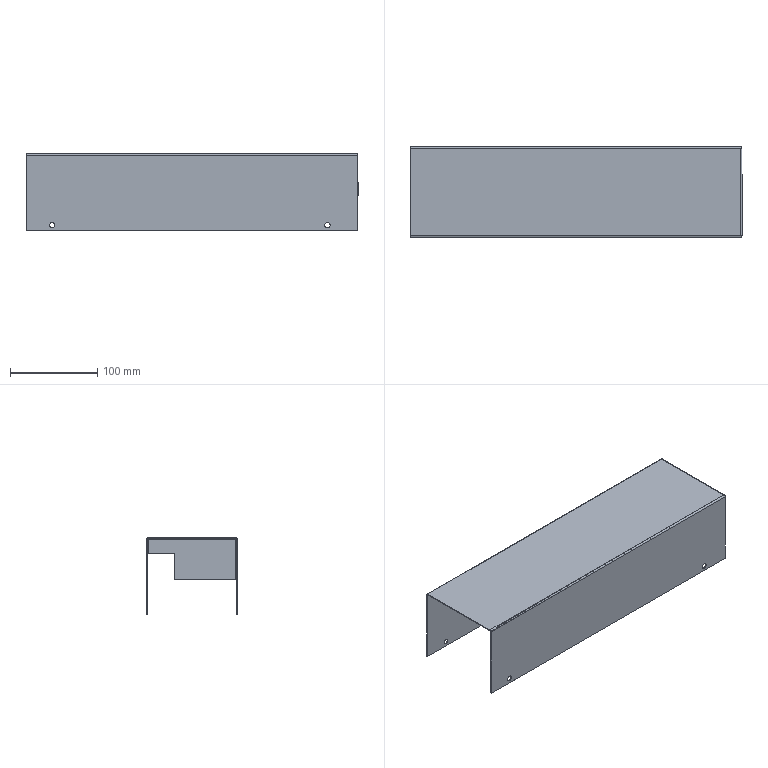Part | SolidWorks | features BaseBody 1 | 1 solid | 38 faces | box 380 x 104 x 88 mm | volume 108125 mm3 | plane 22 | cylinder 16 | commonest cylinder face diameters 6 x8 1.473 x3 3.473 x3 12 x2
STEP:
#1=CARTESIAN_POINT('',(332.,51.,-85.));
#2=VERTEX_POINT('',#1);
#3=CARTESIAN_POINT('',(332.,51.,-79.));
#4=VERTEX_POINT('',#3);
#5=CARTESIAN_POINT('',(332.,51.,-82.));
#6=DIRECTION('',(0.,1.,0.));
#7=DIRECTION('',(0.,0.,1.));
#8=AXIS2_PLACEMENT_3D('',#5,#6,#7);
#9=CIRCLE('',#8,3.);
#10=EDGE_CURVE('',#2,#4,#9,.T.);
#11=ORIENTED_EDGE('',*,*,#10,.F.);
#12=CARTESIAN_POINT('',(332.,52.,-85.));
#13=VERTEX_POINT('',#12);
#14=CARTESIAN_POINT('',(332.,-52.,-85.));
#15=DIRECTION('',(0.,1.,0.));
#16=VECTOR('',#15,1000.);
#17=LINE('',#14,#16);
#18=EDGE_CURVE('',#2,#13,#17,.T.);
#19=ORIENTED_EDGE('',*,*,#18,.T.);
#20=CARTESIAN_POINT('',(332.,52.,-79.));
#21=VERTEX_POINT('',#20);
#22=CARTESIAN_POINT('',(332.,52.,-82.));
#23=DIRECTION('',(0.,1.,0.));
#24=DIRECTION('',(0.,0.,1.));
#25=AXIS2_PLACEMENT_3D('',#22,#23,#24);
#26=CIRCLE('',#25,3.);
#27=EDGE_CURVE('',#13,#21,#26,.T.);
#28=ORIENTED_EDGE('',*,*,#27,.T.);
#29=CARTESIAN_POINT('',(332.,-52.,-79.));
#30=DIRECTION('',(0.,1.,0.));
#31=VECTOR('',#30,1000.);
#32=LINE('',#29,#31);
#33=EDGE_CURVE('',#4,#21,#32,.T.);
#34=ORIENTED_EDGE('',*,*,#33,.F.);
#35=EDGE_LOOP('',(#11,#19,#28,#34));
#36=FACE_OUTER_BOUND('',#35,.T.);
#37=CARTESIAN_POINT('',(332.,-52.,-82.));
#38=DIRECTION('',(0.,1.,0.));
#39=DIRECTION('',(0.,0.,1.));
#40=AXIS2_PLACEMENT_3D('',#37,#38,#39);
#41=CYLINDRICAL_SURFACE('',#40,3.);
#42=ADVANCED_FACE('',(#36),#41,.F.);
#43=CARTESIAN_POINT('',(17.,51.,-85.));
#44=VERTEX_POINT('',#43);
#45=CARTESIAN_POINT('',(17.,51.,-79.));
#46=VERTEX_POINT('',#45);
#47=CARTESIAN_POINT('',(17.,51.,-82.));
#48=DIRECTION('',(0.,1.,0.));
#49=DIRECTION('',(0.,0.,1.));
#50=AXIS2_PLACEMENT_3D('',#47,#48,#49);
#51=CIRCLE('',#50,3.);
#52=EDGE_CURVE('',#44,#46,#51,.T.);
#53=ORIENTED_EDGE('',*,*,#52,.F.);
#54=CARTESIAN_POINT('',(17.,52.,-85.));
#55=VERTEX_POINT('',#54);
#56=CARTESIAN_POINT('',(17.,-52.,-85.));
#57=DIRECTION('',(0.,1.,0.));
#58=VECTOR('',#57,1000.);
#59=LINE('',#56,#58);
#60=EDGE_CURVE('',#44,#55,#59,.T.);
#61=ORIENTED_EDGE('',*,*,#60,.T.);
#62=CARTESIAN_POINT('',(17.,52.,-79.));
#63=VERTEX_POINT('',#62);
#64=CARTESIAN_POINT('',(17.,52.,-82.));
#65=DIRECTION('',(0.,1.,0.));
#66=DIRECTION('',(0.,0.,1.));
#67=AXIS2_PLACEMENT_3D('',#64,#65,#66);
#68=CIRCLE('',#67,3.);
#69=EDGE_CURVE('',#55,#63,#68,.T.);
#70=ORIENTED_EDGE('',*,*,#69,.T.);
#71=CARTESIAN_POINT('',(17.,-52.,-79.));
#72=DIRECTION('',(0.,1.,0.));
#73=VECTOR('',#72,1000.);
#74=LINE('',#71,#73);
#75=EDGE_CURVE('',#46,#63,#74,.T.);
#76=ORIENTED_EDGE('',*,*,#75,.F.);
#77=EDGE_LOOP('',(#53,#61,#70,#76));
#78=FACE_OUTER_BOUND('',#77,.T.);
#79=CARTESIAN_POINT('',(17.,-52.,-82.));
#80=DIRECTION('',(0.,1.,0.));
#81=DIRECTION('',(0.,0.,1.));
#82=AXIS2_PLACEMENT_3D('',#79,#80,#81);
#83=CYLINDRICAL_SURFACE('',#82,3.);
#84=ADVANCED_FACE('',(#78),#83,.F.);
#85=CARTESIAN_POINT('',(17.,-52.,-85.));
#86=VERTEX_POINT('',#85);
#87=CARTESIAN_POINT('',(17.,-52.,-79.));
#88=VERTEX_POINT('',#87);
#89=CARTESIAN_POINT('',(17.,-52.,-82.));
#90=DIRECTION('',(0.,1.,0.));
#91=DIRECTION('',(0.,0.,1.));
#92=AXIS2_PLACEMENT_3D('',#89,#90,#91);
#93=CIRCLE('',#92,3.);
#94=EDGE_CURVE('',#86,#88,#93,.T.);
#95=ORIENTED_EDGE('',*,*,#94,.F.);
#96=CARTESIAN_POINT('',(17.,-51.,-85.));
#97=VERTEX_POINT('',#96);
#98=CARTESIAN_POINT('',(17.,-52.,-85.));
#99=DIRECTION('',(0.,1.,0.));
#100=VECTOR('',#99,1000.);
#101=LINE('',#98,#100);
#102=EDGE_CURVE('',#86,#97,#101,.T.);
#103=ORIENTED_EDGE('',*,*,#102,.T.);
#104=CARTESIAN_POINT('',(17.,-51.,-79.));
#105=VERTEX_POINT('',#104);
#106=CARTESIAN_POINT('',(17.,-51.,-82.));
#107=DIRECTION('',(0.,-1.,0.));
#108=DIRECTION('',(0.,0.,1.));
#109=AXIS2_PLACEMENT_3D('',#106,#107,#108);
#110=CIRCLE('',#109,3.);
#111=EDGE_CURVE('',#105,#97,#110,.T.);
#112=ORIENTED_EDGE('',*,*,#111,.F.);
#113=CARTESIAN_POINT('',(17.,-52.,-79.));
#114=DIRECTION('',(0.,1.,0.));
#115=VECTOR('',#114,1000.);
#116=LINE('',#113,#115);
#117=EDGE_CURVE('',#88,#105,#116,.T.);
#118=ORIENTED_EDGE('',*,*,#117,.F.);
#119=EDGE_LOOP('',(#95,#103,#112,#118));
#120=FACE_OUTER_BOUND('',#119,.T.);
#121=CARTESIAN_POINT('',(17.,-52.,-82.));
#122=DIRECTION('',(0.,1.,0.));
#123=DIRECTION('',(0.,0.,1.));
#124=AXIS2_PLACEMENT_3D('',#121,#122,#123);
#125=CYLINDRICAL_SURFACE('',#124,3.);
#126=ADVANCED_FACE('',(#120),#125,.F.);
#127=CARTESIAN_POINT('',(332.,-52.,-85.));
#128=VERTEX_POINT('',#127);
#129=CARTESIAN_POINT('',(332.,-52.,-79.));
#130=VERTEX_POINT('',#129);
#131=CARTESIAN_POINT('',(332.,-52.,-82.));
#132=DIRECTION('',(0.,1.,0.));
#133=DIRECTION('',(0.,0.,1.));
#134=AXIS2_PLACEMENT_3D('',#131,#132,#133);
#135=CIRCLE('',#134,3.);
#136=EDGE_CURVE('',#128,#130,#135,.T.);
#137=ORIENTED_EDGE('',*,*,#136,.F.);
#138=CARTESIAN_POINT('',(332.,-51.,-85.));
#139=VERTEX_POINT('',#138);
#140=CARTESIAN_POINT('',(332.,-52.,-85.));
#141=DIRECTION('',(0.,1.,0.));
#142=VECTOR('',#141,1000.);
#143=LINE('',#140,#142);
#144=EDGE_CURVE('',#128,#139,#143,.T.);
#145=ORIENTED_EDGE('',*,*,#144,.T.);
#146=CARTESIAN_POINT('',(332.,-51.,-79.));
#147=VERTEX_POINT('',#146);
#148=CARTESIAN_POINT('',(332.,-51.,-82.));
#149=DIRECTION('',(0.,-1.,0.));
#150=DIRECTION('',(0.,0.,1.));
#151=AXIS2_PLACEMENT_3D('',#148,#149,#150);
#152=CIRCLE('',#151,3.);
#153=EDGE_CURVE('',#147,#139,#152,.T.);
#154=ORIENTED_EDGE('',*,*,#153,.F.);
#155=CARTESIAN_POINT('',(332.,-52.,-79.));
#156=DIRECTION('',(0.,1.,0.));
#157=VECTOR('',#156,1000.);
#158=LINE('',#155,#157);
#159=EDGE_CURVE('',#130,#147,#158,.T.);
#160=ORIENTED_EDGE('',*,*,#159,.F.);
#161=EDGE_LOOP('',(#137,#145,#154,#160));
#162=FACE_OUTER_BOUND('',#161,.T.);
#163=CARTESIAN_POINT('',(332.,-52.,-82.));
#164=DIRECTION('',(0.,1.,0.));
#165=DIRECTION('',(0.,0.,1.));
#166=AXIS2_PLACEMENT_3D('',#163,#164,#165);
#167=CYLINDRICAL_SURFACE('',#166,3.);
#168=ADVANCED_FACE('',(#162),#167,.F.);
#169=CARTESIAN_POINT('',(365.263,50.263,0.));
#170=VERTEX_POINT('',#169);
#171=CARTESIAN_POINT('',(-13.,50.263,0.));
#172=VERTEX_POINT('',#171);
#173=CARTESIAN_POINT('',(0.,50.263,0.));
#174=DIRECTION('',(-1.,0.,0.));
#175=VECTOR('',#174,1000.);
#176=LINE('',#173,#175);
#177=EDGE_CURVE('',#170,#172,#176,.T.);
#178=ORIENTED_EDGE('',*,*,#177,.T.);
#179=CARTESIAN_POINT('',(-13.,-50.263,0.));
#180=VERTEX_POINT('',#179);
#181=CARTESIAN_POINT('',(-13.,0.,0.));
#182=DIRECTION('',(0.,-1.,0.));
#183=VECTOR('',#182,1000.);
#184=LINE('',#181,#183);
#185=EDGE_CURVE('',#172,#180,#184,.T.);
#186=ORIENTED_EDGE('',*,*,#185,.T.);
#187=CARTESIAN_POINT('',(365.263,-50.263,0.));
#188=VERTEX_POINT('',#187);
#189=CARTESIAN_POINT('',(0.,-50.263,0.));
#190=DIRECTION('',(1.,0.,0.));
#191=VECTOR('',#190,1000.);
#192=LINE('',#189,#191);
#193=EDGE_CURVE('',#180,#188,#192,.T.);
#194=ORIENTED_EDGE('',*,*,#193,.T.);
#195=CARTESIAN_POINT('',(365.263,0.,0.));
#196=DIRECTION('',(0.,1.,0.));
#197=VECTOR('',#196,1000.);
#198=LINE('',#195,#197);
#199=EDGE_CURVE('',#188,#170,#198,.T.);
#200=ORIENTED_EDGE('',*,*,#199,.T.);
#201=EDGE_LOOP('',(#178,#186,#194,#200));
#202=FACE_OUTER_BOUND('',#201,.T.);
#203=CARTESIAN_POINT('',(0.,0.,0.));
#204=DIRECTION('',(0.,0.,1.));
#205=DIRECTION('',(1.,0.,0.));
#206=AXIS2_PLACEMENT_3D('',#203,#204,#205);
#207=PLANE('',#206);
#208=ADVANCED_FACE('',(#202),#207,.T.);
#209=ORIENTED_EDGE('',*,*,#185,.F.);
#210=CARTESIAN_POINT('',(-13.,52.,-1.737));
#211=VERTEX_POINT('',#210);
#212=CARTESIAN_POINT('',(-13.,50.263,-1.737));
#213=DIRECTION('',(1.,0.,0.));
#214=DIRECTION('',(0.,0.,-1.));
#215=AXIS2_PLACEMENT_3D('',#212,#213,#214);
#216=CIRCLE('',#215,1.737);
#217=EDGE_CURVE('',#211,#172,#216,.T.);
#218=ORIENTED_EDGE('',*,*,#217,.F.);
#219=CARTESIAN_POINT('',(-13.,52.,-88.));
#220=VERTEX_POINT('',#219);
#221=CARTESIAN_POINT('',(-13.,52.,0.));
#222=DIRECTION('',(0.,0.,-1.));
#223=VECTOR('',#222,1000.);
#224=LINE('',#221,#223);
#225=EDGE_CURVE('',#211,#220,#224,.T.);
#226=ORIENTED_EDGE('',*,*,#225,.T.);
#227=CARTESIAN_POINT('',(-13.,51.,-88.));
#228=VERTEX_POINT('',#227);
#229=CARTESIAN_POINT('',(-13.,52.,-88.));
#230=DIRECTION('',(0.,-1.,0.));
#231=VECTOR('',#230,1000.);
#232=LINE('',#229,#231);
#233=EDGE_CURVE('',#220,#228,#232,.T.);
#234=ORIENTED_EDGE('',*,*,#233,.T.);
#235=CARTESIAN_POINT('',(-13.,51.,-1.737));
#236=VERTEX_POINT('',#235);
#237=CARTESIAN_POINT('',(-13.,51.,-1.));
#238=DIRECTION('',(0.,0.,-1.));
#239=VECTOR('',#238,1000.);
#240=LINE('',#237,#239);
#241=EDGE_CURVE('',#236,#228,#240,.T.);
#242=ORIENTED_EDGE('',*,*,#241,.F.);
#243=CARTESIAN_POINT('',(-13.,50.263,-1.));
#244=VERTEX_POINT('',#243);
#245=CARTESIAN_POINT('',(-13.,50.263,-1.737));
#246=DIRECTION('',(1.,0.,0.));
#247=DIRECTION('',(0.,0.,-1.));
#248=AXIS2_PLACEMENT_3D('',#245,#246,#247);
#249=CIRCLE('',#248,0.7366);
#250=EDGE_CURVE('',#236,#244,#249,.T.);
#251=ORIENTED_EDGE('',*,*,#250,.T.);
#252=CARTESIAN_POINT('',(-13.,-50.263,-1.));
#253=VERTEX_POINT('',#252);
#254=CARTESIAN_POINT('',(-13.,51.,-1.));
#255=DIRECTION('',(0.,-1.,0.));
#256=VECTOR('',#255,1000.);
#257=LINE('',#254,#256);
#258=EDGE_CURVE('',#244,#253,#257,.T.);
#259=ORIENTED_EDGE('',*,*,#258,.T.);
#260=CARTESIAN_POINT('',(-13.,-51.,-1.737));
#261=VERTEX_POINT('',#260);
#262=CARTESIAN_POINT('',(-13.,-50.263,-1.737));
#263=DIRECTION('',(-1.,0.,0.));
#264=DIRECTION('',(0.,0.,1.));
#265=AXIS2_PLACEMENT_3D('',#262,#263,#264);
#266=CIRCLE('',#265,0.7366);
#267=EDGE_CURVE('',#261,#253,#266,.T.);
#268=ORIENTED_EDGE('',*,*,#267,.F.);
#269=CARTESIAN_POINT('',(-13.,-51.,-88.));
#270=VERTEX_POINT('',#269);
#271=CARTESIAN_POINT('',(-13.,-51.,-1.));
#272=DIRECTION('',(0.,0.,-1.));
#273=VECTOR('',#272,1000.);
#274=LINE('',#271,#273);
#275=EDGE_CURVE('',#261,#270,#274,.T.);
#276=ORIENTED_EDGE('',*,*,#275,.T.);
#277=CARTESIAN_POINT('',(-13.,-52.,-88.));
#278=VERTEX_POINT('',#277);
#279=CARTESIAN_POINT('',(-13.,-52.,-88.));
#280=DIRECTION('',(0.,1.,0.));
#281=VECTOR('',#280,1000.);
#282=LINE('',#279,#281);
#283=EDGE_CURVE('',#278,#270,#282,.T.);
#284=ORIENTED_EDGE('',*,*,#283,.F.);
#285=CARTESIAN_POINT('',(-13.,-52.,-1.737));
#286=VERTEX_POINT('',#285);
#287=CARTESIAN_POINT('',(-13.,-52.,0.));
#288=DIRECTION('',(0.,0.,-1.));
#289=VECTOR('',#288,1000.);
#290=LINE('',#287,#289);
#291=EDGE_CURVE('',#286,#278,#290,.T.);
#292=ORIENTED_EDGE('',*,*,#291,.F.);
#293=CARTESIAN_POINT('',(-13.,-50.263,-1.737));
#294=DIRECTION('',(1.,0.,0.));
#295=DIRECTION('',(0.,0.,1.));
#296=AXIS2_PLACEMENT_3D('',#293,#294,#295);
#297=CIRCLE('',#296,1.737);
#298=EDGE_CURVE('',#180,#286,#297,.T.);
#299=ORIENTED_EDGE('',*,*,#298,.F.);
#300=EDGE_LOOP('',(#209,#218,#226,#234,#242,#251,#259,#268,#276,#284,#292,#299));
#301=FACE_OUTER_BOUND('',#300,.T.);
#302=CARTESIAN_POINT('',(-13.,51.,-1.));
#303=DIRECTION('',(-1.,0.,0.));
#304=DIRECTION('',(0.,0.,1.));
#305=AXIS2_PLACEMENT_3D('',#302,#303,#304);
#306=PLANE('',#305);
#307=ADVANCED_FACE('',(#301),#306,.T.);
#308=ORIENTED_EDGE('',*,*,#217,.T.);
#309=ORIENTED_EDGE('',*,*,#177,.F.);
#310=CARTESIAN_POINT('',(366.,50.263,0.));
#311=VERTEX_POINT('',#310);
#312=CARTESIAN_POINT('',(366.,50.263,0.));
#313=DIRECTION('',(1.,0.,0.));
#314=VECTOR('',#313,1000.);
#315=LINE('',#312,#314);
#316=EDGE_CURVE('',#170,#311,#315,.T.);
#317=ORIENTED_EDGE('',*,*,#316,.T.);
#318=CARTESIAN_POINT('',(366.,52.,-1.737));
#319=VERTEX_POINT('',#318);
#320=CARTESIAN_POINT('',(366.,50.263,-1.737));
#321=DIRECTION('',(-1.,0.,0.));
#322=DIRECTION('',(0.,0.,-1.));
#323=AXIS2_PLACEMENT_3D('',#320,#321,#322);
#324=CIRCLE('',#323,1.737);
#325=EDGE_CURVE('',#311,#319,#324,.T.);
#326=ORIENTED_EDGE('',*,*,#325,.T.);
#327=CARTESIAN_POINT('',(366.,52.,-1.737));
#328=DIRECTION('',(-1.,0.,0.));
#329=VECTOR('',#328,1000.);
#330=LINE('',#327,#329);
#331=EDGE_CURVE('',#319,#211,#330,.T.);
#332=ORIENTED_EDGE('',*,*,#331,.T.);
#333=EDGE_LOOP('',(#308,#309,#317,#326,#332));
#334=FACE_OUTER_BOUND('',#333,.T.);
#335=CARTESIAN_POINT('',(366.,50.263,-1.737));
#336=DIRECTION('',(1.,0.,0.));
#337=DIRECTION('',(0.,0.,-1.));
#338=AXIS2_PLACEMENT_3D('',#335,#336,#337);
#339=CYLINDRICAL_SURFACE('',#338,1.737);
#340=ADVANCED_FACE('',(#334),#339,.T.);
#341=CARTESIAN_POINT('',(367.,50.263,-1.737));
#342=VERTEX_POINT('',#341);
#343=CARTESIAN_POINT('',(366.,50.263,-0.164));
#344=VERTEX_POINT('',#343);
#345=CARTESIAN_POINT('',(365.263,50.263,-1.737));
#346=DIRECTION('',(0.,-1.,0.));
#347=DIRECTION('',(0.,0.,-1.));
#348=AXIS2_PLACEMENT_3D('',#345,#346,#347);
#349=CIRCLE('',#348,1.737);
#350=EDGE_CURVE('',#342,#344,#349,.T.);
#351=ORIENTED_EDGE('',*,*,#350,.T.);
#352=CARTESIAN_POINT('',(365.263,50.263,-1.737));
#353=DIRECTION('',(0.,-1.,0.));
#354=DIRECTION('',(0.,0.,-1.));
#355=AXIS2_PLACEMENT_3D('',#352,#353,#354);
#356=CIRCLE('',#355,1.737);
#357=EDGE_CURVE('',#344,#170,#356,.T.);
#358=ORIENTED_EDGE('',*,*,#357,.T.);
#359=ORIENTED_EDGE('',*,*,#199,.F.);
#360=CARTESIAN_POINT('',(366.,-50.263,-0.164));
#361=VERTEX_POINT('',#360);
#362=CARTESIAN_POINT('',(365.263,-50.263,-1.737));
#363=DIRECTION('',(0.,1.,0.));
#364=DIRECTION('',(0.,0.,-1.));
#365=AXIS2_PLACEMENT_3D('',#362,#363,#364);
#366=CIRCLE('',#365,1.737);
#367=EDGE_CURVE('',#188,#361,#366,.T.);
#368=ORIENTED_EDGE('',*,*,#367,.T.);
#369=CARTESIAN_POINT('',(367.,-50.263,-1.737));
#370=VERTEX_POINT('',#369);
#371=CARTESIAN_POINT('',(365.263,-50.263,-1.737));
#372=DIRECTION('',(0.,1.,0.));
#373=DIRECTION('',(0.,0.,-1.));
#374=AXIS2_PLACEMENT_3D('',#371,#372,#373);
#375=CIRCLE('',#374,1.737);
#376=EDGE_CURVE('',#361,#370,#375,.T.);
#377=ORIENTED_EDGE('',*,*,#376,.T.);
#378=CARTESIAN_POINT('',(367.,-50.263,-1.737));
#379=DIRECTION('',(0.,1.,0.));
#380=VECTOR('',#379,1000.);
#381=LINE('',#378,#380);
#382=EDGE_CURVE('',#370,#342,#381,.T.);
#383=ORIENTED_EDGE('',*,*,#382,.T.);
#384=EDGE_LOOP('',(#351,#358,#359,#368,#377,#383));
#385=FACE_OUTER_BOUND('',#384,.T.);
#386=CARTESIAN_POINT('',(365.263,-50.263,-1.737));
#387=DIRECTION('',(0.,-1.,0.));
#388=DIRECTION('',(0.,0.,-1.));
#389=AXIS2_PLACEMENT_3D('',#386,#387,#388);
#390=CYLINDRICAL_SURFACE('',#389,1.737);
#391=ADVANCED_FACE('',(#385),#390,.T.);
#392=CARTESIAN_POINT('',(366.,-52.,-1.737));
#393=VERTEX_POINT('',#392);
#394=CARTESIAN_POINT('',(366.,-50.263,0.));
#395=VERTEX_POINT('',#394);
#396=CARTESIAN_POINT('',(366.,-50.263,-1.737));
#397=DIRECTION('',(-1.,0.,0.));
#398=DIRECTION('',(0.,0.,1.));
#399=AXIS2_PLACEMENT_3D('',#396,#397,#398);
#400=CIRCLE('',#399,1.737);
#401=EDGE_CURVE('',#393,#395,#400,.T.);
#402=ORIENTED_EDGE('',*,*,#401,.T.);
#403=CARTESIAN_POINT('',(-13.,-50.263,0.));
#404=DIRECTION('',(-1.,0.,0.));
#405=VECTOR('',#404,1000.);
#406=LINE('',#403,#405);
#407=EDGE_CURVE('',#395,#188,#406,.T.);
#408=ORIENTED_EDGE('',*,*,#407,.T.);
#409=ORIENTED_EDGE('',*,*,#193,.F.);
#410=ORIENTED_EDGE('',*,*,#298,.T.);
#411=CARTESIAN_POINT('',(-13.,-52.,-1.737));
#412=DIRECTION('',(1.,0.,0.));
#413=VECTOR('',#412,1000.);
#414=LINE('',#411,#413);
#415=EDGE_CURVE('',#286,#393,#414,.T.);
#416=ORIENTED_EDGE('',*,*,#415,.T.);
#417=EDGE_LOOP('',(#402,#408,#409,#410,#416));
#418=FACE_OUTER_BOUND('',#417,.T.);
#419=CARTESIAN_POINT('',(-13.,-50.263,-1.737));
#420=DIRECTION('',(-1.,0.,0.));
#421=DIRECTION('',(0.,0.,1.));
#422=AXIS2_PLACEMENT_3D('',#419,#420,#421);
#423=CYLINDRICAL_SURFACE('',#422,1.737);
#424=ADVANCED_FACE('',(#418),#423,.T.);
#425=CARTESIAN_POINT('',(365.263,-50.263,-1.));
#426=VERTEX_POINT('',#425);
#427=CARTESIAN_POINT('',(0.,-50.263,-1.));
#428=DIRECTION('',(1.,0.,0.));
#429=VECTOR('',#428,1000.);
#430=LINE('',#427,#429);
#431=EDGE_CURVE('',#253,#426,#430,.T.);
#432=ORIENTED_EDGE('',*,*,#431,.F.);
#433=ORIENTED_EDGE('',*,*,#258,.F.);
#434=CARTESIAN_POINT('',(365.263,50.263,-1.));
#435=VERTEX_POINT('',#434);
#436=CARTESIAN_POINT('',(0.,50.263,-1.));
#437=DIRECTION('',(-1.,0.,0.));
#438=VECTOR('',#437,1000.);
#439=LINE('',#436,#438);
#440=EDGE_CURVE('',#435,#244,#439,.T.);
#441=ORIENTED_EDGE('',*,*,#440,.F.);
#442=CARTESIAN_POINT('',(365.263,0.,-1.));
#443=DIRECTION('',(0.,1.,0.));
#444=VECTOR('',#443,1000.);
#445=LINE('',#442,#444);
#446=EDGE_CURVE('',#426,#435,#445,.T.);
#447=ORIENTED_EDGE('',*,*,#446,.F.);
#448=EDGE_LOOP('',(#432,#433,#441,#447));
#449=FACE_OUTER_BOUND('',#448,.T.);
#450=CARTESIAN_POINT('',(0.,0.,-1.));
#451=DIRECTION('',(0.,0.,1.));
#452=DIRECTION('',(1.,0.,0.));
#453=AXIS2_PLACEMENT_3D('',#450,#451,#452);
#454=PLANE('',#453);
#455=ADVANCED_FACE('',(#449),#454,.F.);
#456=CARTESIAN_POINT('',(246.,52.,-32.));
#457=VERTEX_POINT('',#456);
#458=CARTESIAN_POINT('',(246.,52.,-44.));
#459=VERTEX_POINT('',#458);
#460=CARTESIAN_POINT('',(246.,52.,-38.));
#461=DIRECTION('',(0.,1.,0.));
#462=DIRECTION('',(0.,0.,1.));
#463=AXIS2_PLACEMENT_3D('',#460,#461,#462);
#464=CIRCLE('',#463,6.);
#465=EDGE_CURVE('',#457,#459,#464,.T.);
#466=ORIENTED_EDGE('',*,*,#465,.F.);
#467=CARTESIAN_POINT('',(206.,52.,-32.));
#468=VERTEX_POINT('',#467);
#469=CARTESIAN_POINT('',(0.,52.,-32.));
#470=DIRECTION('',(1.,0.,0.));
#471=VECTOR('',#470,1000.);
#472=LINE('',#469,#471);
#473=EDGE_CURVE('',#468,#457,#472,.T.);
#474=ORIENTED_EDGE('',*,*,#473,.F.);
#475=CARTESIAN_POINT('',(206.,52.,-44.));
#476=VERTEX_POINT('',#475);
#477=CARTESIAN_POINT('',(206.,52.,-38.));
#478=DIRECTION('',(0.,1.,0.));
#479=DIRECTION('',(0.,0.,-1.));
#480=AXIS2_PLACEMENT_3D('',#477,#478,#479);
#481=CIRCLE('',#480,6.);
#482=EDGE_CURVE('',#476,#468,#481,.T.);
#483=ORIENTED_EDGE('',*,*,#482,.F.);
#484=CARTESIAN_POINT('',(0.,52.,-44.));
#485=DIRECTION('',(-1.,0.,0.));
#486=VECTOR('',#485,1000.);
#487=LINE('',#484,#486);
#488=EDGE_CURVE('',#459,#476,#487,.T.);
#489=ORIENTED_EDGE('',*,*,#488,.F.);
#490=EDGE_LOOP('',(#466,#474,#483,#489));
#491=FACE_BOUND('',#490,.T.);
#492=CARTESIAN_POINT('',(332.,52.,-82.));
#493=DIRECTION('',(0.,1.,0.));
#494=DIRECTION('',(0.,0.,1.));
#495=AXIS2_PLACEMENT_3D('',#492,#493,#494);
#496=CIRCLE('',#495,3.);
#497=EDGE_CURVE('',#21,#13,#496,.T.);
#498=ORIENTED_EDGE('',*,*,#497,.F.);
#499=ORIENTED_EDGE('',*,*,#27,.F.);
#500=EDGE_LOOP('',(#498,#499));
#501=FACE_BOUND('',#500,.T.);
#502=CARTESIAN_POINT('',(17.,52.,-82.));
#503=DIRECTION('',(0.,1.,0.));
#504=DIRECTION('',(0.,0.,1.));
#505=AXIS2_PLACEMENT_3D('',#502,#503,#504);
#506=CIRCLE('',#505,3.);
#507=EDGE_CURVE('',#63,#55,#506,.T.);
#508=ORIENTED_EDGE('',*,*,#507,.F.);
#509=ORIENTED_EDGE('',*,*,#69,.F.);
#510=EDGE_LOOP('',(#508,#509));
#511=FACE_BOUND('',#510,.T.);
#512=CARTESIAN_POINT('',(366.,52.,-88.));
#513=VERTEX_POINT('',#512);
#514=CARTESIAN_POINT('',(366.,52.,0.));
#515=DIRECTION('',(0.,0.,1.));
#516=VECTOR('',#515,1000.);
#517=LINE('',#514,#516);
#518=EDGE_CURVE('',#513,#319,#517,.T.);
#519=ORIENTED_EDGE('',*,*,#518,.F.);
#520=CARTESIAN_POINT('',(0.,52.,-88.));
#521=DIRECTION('',(1.,0.,0.));
#522=VECTOR('',#521,1000.);
#523=LINE('',#520,#522);
#524=EDGE_CURVE('',#220,#513,#523,.T.);
#525=ORIENTED_EDGE('',*,*,#524,.F.);
#526=ORIENTED_EDGE('',*,*,#225,.F.);
#527=ORIENTED_EDGE('',*,*,#331,.F.);
#528=EDGE_LOOP('',(#519,#525,#526,#527));
#529=FACE_OUTER_BOUND('',#528,.T.);
#530=CARTESIAN_POINT('',(0.,52.,0.));
#531=DIRECTION('',(0.,-1.,0.));
#532=DIRECTION('',(0.,0.,-1.));
#533=AXIS2_PLACEMENT_3D('',#530,#531,#532);
#534=PLANE('',#533);
#535=ADVANCED_FACE('',(#491,#501,#511,#529),#534,.F.);
#536=CARTESIAN_POINT('',(366.,51.,-1.737));
#537=VERTEX_POINT('',#536);
#538=CARTESIAN_POINT('',(366.,50.263,-1.));
#539=VERTEX_POINT('',#538);
#540=CARTESIAN_POINT('',(366.,50.263,-1.737));
#541=DIRECTION('',(1.,0.,0.));
#542=DIRECTION('',(0.,0.,-1.));
#543=AXIS2_PLACEMENT_3D('',#540,#541,#542);
#544=CIRCLE('',#543,0.7366);
#545=EDGE_CURVE('',#537,#539,#544,.T.);
#546=ORIENTED_EDGE('',*,*,#545,.F.);
#547=CARTESIAN_POINT('',(366.,51.,-88.));
#548=VERTEX_POINT('',#547);
#549=CARTESIAN_POINT('',(366.,51.,-88.));
#550=DIRECTION('',(0.,0.,1.));
#551=VECTOR('',#550,1000.);
#552=LINE('',#549,#551);
#553=EDGE_CURVE('',#548,#537,#552,.T.);
#554=ORIENTED_EDGE('',*,*,#553,.F.);
#555=CARTESIAN_POINT('',(366.,52.,-88.));
#556=DIRECTION('',(0.,-1.,0.));
#557=VECTOR('',#556,1000.);
#558=LINE('',#555,#557);
#559=EDGE_CURVE('',#513,#548,#558,.T.);
#560=ORIENTED_EDGE('',*,*,#559,.F.);
#561=ORIENTED_EDGE('',*,*,#518,.T.);
#562=ORIENTED_EDGE('',*,*,#325,.F.);
#563=CARTESIAN_POINT('',(366.,50.263,-1.737));
#564=DIRECTION('',(0.,0.,1.));
#565=VECTOR('',#564,1000.);
#566=LINE('',#563,#565);
#567=EDGE_CURVE('',#344,#311,#566,.T.);
#568=ORIENTED_EDGE('',*,*,#567,.F.);
#569=CARTESIAN_POINT('',(366.,50.263,-1.737));
#570=DIRECTION('',(0.,0.,1.));
#571=VECTOR('',#570,1000.);
#572=LINE('',#569,#571);
#573=EDGE_CURVE('',#539,#344,#572,.T.);
#574=ORIENTED_EDGE('',*,*,#573,.F.);
#575=EDGE_LOOP('',(#546,#554,#560,#561,#562,#568,#574));
#576=FACE_OUTER_BOUND('',#575,.T.);
#577=CARTESIAN_POINT('',(366.,50.263,-1.737));
#578=DIRECTION('',(-1.,0.,0.));
#579=DIRECTION('',(0.,0.,1.));
#580=AXIS2_PLACEMENT_3D('',#577,#578,#579);
#581=PLANE('',#580);
#582=ADVANCED_FACE('',(#576),#581,.F.);
#583=ORIENTED_EDGE('',*,*,#357,.F.);
#584=ORIENTED_EDGE('',*,*,#567,.T.);
#585=ORIENTED_EDGE('',*,*,#316,.F.);
#586=EDGE_LOOP('',(#583,#584,#585));
#587=FACE_OUTER_BOUND('',#586,.T.);
#588=CARTESIAN_POINT('',(365.263,50.263,-1.));
#589=DIRECTION('',(0.,-1.,0.));
#590=DIRECTION('',(0.,0.,-1.));
#591=AXIS2_PLACEMENT_3D('',#588,#589,#590);
#592=PLANE('',#591);
#593=ADVANCED_FACE('',(#587),#592,.T.);
#594=ORIENTED_EDGE('',*,*,#350,.F.);
#595=CARTESIAN_POINT('',(367.,50.263,-18.));
#596=VERTEX_POINT('',#595);
#597=CARTESIAN_POINT('',(367.,50.263,0.));
#598=DIRECTION('',(0.,0.,1.));
#599=VECTOR('',#598,1000.);
#600=LINE('',#597,#599);
#601=EDGE_CURVE('',#596,#342,#600,.T.);
#602=ORIENTED_EDGE('',*,*,#601,.F.);
#603=CARTESIAN_POINT('',(366.,50.263,-18.));
#604=VERTEX_POINT('',#603);
#605=CARTESIAN_POINT('',(367.,50.263,-18.));
#606=DIRECTION('',(-1.,0.,0.));
#607=VECTOR('',#606,1000.);
#608=LINE('',#605,#607);
#609=EDGE_CURVE('',#596,#604,#608,.T.);
#610=ORIENTED_EDGE('',*,*,#609,.T.);
#611=CARTESIAN_POINT('',(366.,50.263,-1.737));
#612=VERTEX_POINT('',#611);
#613=CARTESIAN_POINT('',(366.,50.263,-48.));
#614=DIRECTION('',(0.,0.,1.));
#615=VECTOR('',#614,1000.);
#616=LINE('',#613,#615);
#617=EDGE_CURVE('',#604,#612,#616,.T.);
#618=ORIENTED_EDGE('',*,*,#617,.T.);
#619=CARTESIAN_POINT('',(365.263,50.263,-1.737));
#620=DIRECTION('',(0.,-1.,0.));
#621=DIRECTION('',(0.,0.,-1.));
#622=AXIS2_PLACEMENT_3D('',#619,#620,#621);
#623=CIRCLE('',#622,0.7366);
#624=EDGE_CURVE('',#612,#435,#623,.T.);
#625=ORIENTED_EDGE('',*,*,#624,.T.);
#626=CARTESIAN_POINT('',(365.263,50.263,-1.));
#627=DIRECTION('',(1.,0.,0.));
#628=VECTOR('',#627,1000.);
#629=LINE('',#626,#628);
#630=EDGE_CURVE('',#435,#539,#629,.T.);
#631=ORIENTED_EDGE('',*,*,#630,.T.);
#632=ORIENTED_EDGE('',*,*,#573,.T.);
#633=EDGE_LOOP('',(#594,#602,#610,#618,#625,#631,#632));
#634=FACE_OUTER_BOUND('',#633,.T.);
#635=CARTESIAN_POINT('',(365.263,50.263,-1.737));
#636=DIRECTION('',(0.,1.,0.));
#637=DIRECTION('',(0.,0.,1.));
#638=AXIS2_PLACEMENT_3D('',#635,#636,#637);
#639=PLANE('',#638);
#640=ADVANCED_FACE('',(#634),#639,.T.);
#641=CARTESIAN_POINT('',(367.,-50.263,-48.));
#642=VERTEX_POINT('',#641);
#643=CARTESIAN_POINT('',(367.,-50.263,0.));
#644=DIRECTION('',(0.,0.,-1.));
#645=VECTOR('',#644,1000.);
#646=LINE('',#643,#645);
#647=EDGE_CURVE('',#370,#642,#646,.T.);
#648=ORIENTED_EDGE('',*,*,#647,.T.);
#649=CARTESIAN_POINT('',(367.,20.263,-48.));
#650=VERTEX_POINT('',#649);
#651=CARTESIAN_POINT('',(367.,0.,-48.));
#652=DIRECTION('',(0.,1.,0.));
#653=VECTOR('',#652,1000.);
#654=LINE('',#651,#653);
#655=EDGE_CURVE('',#642,#650,#654,.T.);
#656=ORIENTED_EDGE('',*,*,#655,.T.);
#657=CARTESIAN_POINT('',(367.,20.263,-18.));
#658=VERTEX_POINT('',#657);
#659=CARTESIAN_POINT('',(367.,20.263,0.));
#660=DIRECTION('',(0.,0.,1.));
#661=VECTOR('',#660,1000.);
#662=LINE('',#659,#661);
#663=EDGE_CURVE('',#650,#658,#662,.T.);
#664=ORIENTED_EDGE('',*,*,#663,.T.);
#665=CARTESIAN_POINT('',(367.,0.,-18.));
#666=DIRECTION('',(0.,1.,0.));
#667=VECTOR('',#666,1000.);
#668=LINE('',#665,#667);
#669=EDGE_CURVE('',#658,#596,#668,.T.);
#670=ORIENTED_EDGE('',*,*,#669,.T.);
#671=ORIENTED_EDGE('',*,*,#601,.T.);
#672=ORIENTED_EDGE('',*,*,#382,.F.);
#673=EDGE_LOOP('',(#648,#656,#664,#670,#671,#672));
#674=FACE_OUTER_BOUND('',#673,.T.);
#675=CARTESIAN_POINT('',(367.,0.,0.));
#676=DIRECTION('',(1.,0.,0.));
#677=DIRECTION('',(0.,0.,-1.));
#678=AXIS2_PLACEMENT_3D('',#675,#676,#677);
#679=PLANE('',#678);
#680=ADVANCED_FACE('',(#674),#679,.T.);
#681=CARTESIAN_POINT('',(366.,-50.263,-1.));
#682=VERTEX_POINT('',#681);
#683=CARTESIAN_POINT('',(365.263,-50.263,-1.));
#684=DIRECTION('',(1.,0.,0.));
#685=VECTOR('',#684,1000.);
#686=LINE('',#683,#685);
#687=EDGE_CURVE('',#426,#682,#686,.T.);
#688=ORIENTED_EDGE('',*,*,#687,.F.);
#689=CARTESIAN_POINT('',(366.,-50.263,-1.737));
#690=VERTEX_POINT('',#689);
#691=CARTESIAN_POINT('',(365.263,-50.263,-1.737));
#692=DIRECTION('',(0.,-1.,0.));
#693=DIRECTION('',(0.,0.,-1.));
#694=AXIS2_PLACEMENT_3D('',#691,#692,#693);
#695=CIRCLE('',#694,0.7366);
#696=EDGE_CURVE('',#690,#426,#695,.T.);
#697=ORIENTED_EDGE('',*,*,#696,.F.);
#698=CARTESIAN_POINT('',(366.,-50.263,-48.));
#699=VERTEX_POINT('',#698);
#700=CARTESIAN_POINT('',(366.,-50.263,-1.));
#701=DIRECTION('',(0.,0.,-1.));
#702=VECTOR('',#701,1000.);
#703=LINE('',#700,#702);
#704=EDGE_CURVE('',#690,#699,#703,.T.);
#705=ORIENTED_EDGE('',*,*,#704,.T.);
#706=CARTESIAN_POINT('',(367.,-50.263,-48.));
#707=DIRECTION('',(-1.,0.,0.));
#708=VECTOR('',#707,1000.);
#709=LINE('',#706,#708);
#710=EDGE_CURVE('',#642,#699,#709,.T.);
#711=ORIENTED_EDGE('',*,*,#710,.F.);
#712=ORIENTED_EDGE('',*,*,#647,.F.);
#713=ORIENTED_EDGE('',*,*,#376,.F.);
#714=CARTESIAN_POINT('',(366.,-50.263,-1.737));
#715=DIRECTION('',(0.,0.,1.));
#716=VECTOR('',#715,1000.);
#717=LINE('',#714,#716);
#718=EDGE_CURVE('',#682,#361,#717,.T.);
#719=ORIENTED_EDGE('',*,*,#718,.F.);
#720=EDGE_LOOP('',(#688,#697,#705,#711,#712,#713,#719));
#721=FACE_OUTER_BOUND('',#720,.T.);
#722=CARTESIAN_POINT('',(365.263,-50.263,-1.737));
#723=DIRECTION('',(0.,1.,0.));
#724=DIRECTION('',(0.,0.,1.));
#725=AXIS2_PLACEMENT_3D('',#722,#723,#724);
#726=PLANE('',#725);
#727=ADVANCED_FACE('',(#721),#726,.F.);
#728=ORIENTED_EDGE('',*,*,#367,.F.);
#729=ORIENTED_EDGE('',*,*,#407,.F.);
#730=CARTESIAN_POINT('',(366.,-50.263,-1.));
#731=DIRECTION('',(0.,0.,-1.));
#732=VECTOR('',#731,1000.);
#733=LINE('',#730,#732);
#734=EDGE_CURVE('',#395,#361,#733,.T.);
#735=ORIENTED_EDGE('',*,*,#734,.T.);
#736=EDGE_LOOP('',(#728,#729,#735));
#737=FACE_OUTER_BOUND('',#736,.T.);
#738=CARTESIAN_POINT('',(366.,-50.263,-1.));
#739=DIRECTION('',(0.,1.,0.));
#740=DIRECTION('',(0.,0.,1.));
#741=AXIS2_PLACEMENT_3D('',#738,#739,#740);
#742=PLANE('',#741);
#743=ADVANCED_FACE('',(#737),#742,.T.);
#744=ORIENTED_EDGE('',*,*,#734,.F.);
#745=ORIENTED_EDGE('',*,*,#401,.F.);
#746=CARTESIAN_POINT('',(366.,-52.,-88.));
#747=VERTEX_POINT('',#746);
#748=CARTESIAN_POINT('',(366.,-52.,0.));
#749=DIRECTION('',(0.,0.,1.));
#750=VECTOR('',#749,1000.);
#751=LINE('',#748,#750);
#752=EDGE_CURVE('',#747,#393,#751,.T.);
#753=ORIENTED_EDGE('',*,*,#752,.F.);
#754=CARTESIAN_POINT('',(366.,-51.,-88.));
#755=VERTEX_POINT('',#754);
#756=CARTESIAN_POINT('',(366.,-52.,-88.));
#757=DIRECTION('',(0.,-1.,0.));
#758=VECTOR('',#757,1000.);
#759=LINE('',#756,#758);
#760=EDGE_CURVE('',#755,#747,#759,.T.);
#761=ORIENTED_EDGE('',*,*,#760,.F.);
#762=CARTESIAN_POINT('',(366.,-51.,-1.737));
#763=VERTEX_POINT('',#762);
#764=CARTESIAN_POINT('',(366.,-51.,-88.));
#765=DIRECTION('',(0.,0.,1.));
#766=VECTOR('',#765,1000.);
#767=LINE('',#764,#766);
#768=EDGE_CURVE('',#755,#763,#767,.T.);
#769=ORIENTED_EDGE('',*,*,#768,.T.);
#770=CARTESIAN_POINT('',(366.,-50.263,-1.737));
#771=DIRECTION('',(-1.,0.,0.));
#772=DIRECTION('',(0.,0.,1.));
#773=AXIS2_PLACEMENT_3D('',#770,#771,#772);
#774=CIRCLE('',#773,0.7366);
#775=EDGE_CURVE('',#763,#682,#774,.T.);
#776=ORIENTED_EDGE('',*,*,#775,.T.);
#777=ORIENTED_EDGE('',*,*,#718,.T.);
#778=EDGE_LOOP('',(#744,#745,#753,#761,#769,#776,#777));
#779=FACE_OUTER_BOUND('',#778,.T.);
#780=CARTESIAN_POINT('',(366.,-50.263,-1.737));
#781=DIRECTION('',(1.,0.,0.));
#782=DIRECTION('',(0.,0.,-1.));
#783=AXIS2_PLACEMENT_3D('',#780,#781,#782);
#784=PLANE('',#783);
#785=ADVANCED_FACE('',(#779),#784,.T.);
#786=ORIENTED_EDGE('',*,*,#291,.T.);
#787=CARTESIAN_POINT('',(0.,-52.,-88.));
#788=DIRECTION('',(1.,0.,0.));
#789=VECTOR('',#788,1000.);
#790=LINE('',#787,#789);
#791=EDGE_CURVE('',#278,#747,#790,.T.);
#792=ORIENTED_EDGE('',*,*,#791,.T.);
#793=ORIENTED_EDGE('',*,*,#752,.T.);
#794=ORIENTED_EDGE('',*,*,#415,.F.);
#795=EDGE_LOOP('',(#786,#792,#793,#794));
#796=FACE_OUTER_BOUND('',#795,.T.);
#797=CARTESIAN_POINT('',(17.,-52.,-82.));
#798=DIRECTION('',(0.,1.,0.));
#799=DIRECTION('',(0.,0.,1.));
#800=AXIS2_PLACEMENT_3D('',#797,#798,#799);
#801=CIRCLE('',#800,3.);
#802=EDGE_CURVE('',#88,#86,#801,.T.);
#803=ORIENTED_EDGE('',*,*,#802,.T.);
#804=ORIENTED_EDGE('',*,*,#94,.T.);
#805=EDGE_LOOP('',(#803,#804));
#806=FACE_BOUND('',#805,.T.);
#807=CARTESIAN_POINT('',(332.,-52.,-82.));
#808=DIRECTION('',(0.,1.,0.));
#809=DIRECTION('',(0.,0.,1.));
#810=AXIS2_PLACEMENT_3D('',#807,#808,#809);
#811=CIRCLE('',#810,3.);
#812=EDGE_CURVE('',#130,#128,#811,.T.);
#813=ORIENTED_EDGE('',*,*,#812,.T.);
#814=ORIENTED_EDGE('',*,*,#136,.T.);
#815=EDGE_LOOP('',(#813,#814));
#816=FACE_BOUND('',#815,.T.);
#817=CARTESIAN_POINT('',(0.,-52.,0.));
#818=DIRECTION('',(0.,-1.,0.));
#819=DIRECTION('',(0.,0.,-1.));
#820=AXIS2_PLACEMENT_3D('',#817,#818,#819);
#821=PLANE('',#820);
#822=ADVANCED_FACE('',(#796,#806,#816),#821,.T.);
#823=ORIENTED_EDGE('',*,*,#624,.F.);
#824=CARTESIAN_POINT('',(366.,-50.263,-1.737));
#825=DIRECTION('',(0.,1.,0.));
#826=VECTOR('',#825,1000.);
#827=LINE('',#824,#826);
#828=EDGE_CURVE('',#690,#612,#827,.T.);
#829=ORIENTED_EDGE('',*,*,#828,.F.);
#830=ORIENTED_EDGE('',*,*,#696,.T.);
#831=ORIENTED_EDGE('',*,*,#446,.T.);
#832=EDGE_LOOP('',(#823,#829,#830,#831));
#833=FACE_OUTER_BOUND('',#832,.T.);
#834=CARTESIAN_POINT('',(365.263,-50.263,-1.737));
#835=DIRECTION('',(0.,-1.,0.));
#836=DIRECTION('',(0.,0.,-1.));
#837=AXIS2_PLACEMENT_3D('',#834,#835,#836);
#838=CYLINDRICAL_SURFACE('',#837,0.7366);
#839=ADVANCED_FACE('',(#833),#838,.F.);
#840=ORIENTED_EDGE('',*,*,#687,.T.);
#841=ORIENTED_EDGE('',*,*,#775,.F.);
#842=CARTESIAN_POINT('',(-13.,-51.,-1.737));
#843=DIRECTION('',(1.,0.,0.));
#844=VECTOR('',#843,1000.);
#845=LINE('',#842,#844);
#846=EDGE_CURVE('',#261,#763,#845,.T.);
#847=ORIENTED_EDGE('',*,*,#846,.F.);
#848=ORIENTED_EDGE('',*,*,#267,.T.);
#849=ORIENTED_EDGE('',*,*,#431,.T.);
#850=EDGE_LOOP('',(#840,#841,#847,#848,#849));
#851=FACE_OUTER_BOUND('',#850,.T.);
#852=CARTESIAN_POINT('',(-13.,-50.263,-1.737));
#853=DIRECTION('',(-1.,0.,0.));
#854=DIRECTION('',(0.,0.,1.));
#855=AXIS2_PLACEMENT_3D('',#852,#853,#854);
#856=CYLINDRICAL_SURFACE('',#855,0.7366);
#857=ADVANCED_FACE('',(#851),#856,.F.);
#858=ORIENTED_EDGE('',*,*,#440,.T.);
#859=ORIENTED_EDGE('',*,*,#250,.F.);
#860=CARTESIAN_POINT('',(366.,51.,-1.737));
#861=DIRECTION('',(-1.,0.,0.));
#862=VECTOR('',#861,1000.);
#863=LINE('',#860,#862);
#864=EDGE_CURVE('',#537,#236,#863,.T.);
#865=ORIENTED_EDGE('',*,*,#864,.F.);
#866=ORIENTED_EDGE('',*,*,#545,.T.);
#867=ORIENTED_EDGE('',*,*,#630,.F.);
#868=EDGE_LOOP('',(#858,#859,#865,#866,#867));
#869=FACE_OUTER_BOUND('',#868,.T.);
#870=CARTESIAN_POINT('',(366.,50.263,-1.737));
#871=DIRECTION('',(1.,0.,0.));
#872=DIRECTION('',(0.,0.,-1.));
#873=AXIS2_PLACEMENT_3D('',#870,#871,#872);
#874=CYLINDRICAL_SURFACE('',#873,0.7366);
#875=ADVANCED_FACE('',(#869),#874,.F.);
#876=CARTESIAN_POINT('',(246.,51.,-44.));
#877=VERTEX_POINT('',#876);
#878=CARTESIAN_POINT('',(206.,51.,-44.));
#879=VERTEX_POINT('',#878);
#880=CARTESIAN_POINT('',(0.,51.,-44.));
#881=DIRECTION('',(-1.,0.,0.));
#882=VECTOR('',#881,1000.);
#883=LINE('',#880,#882);
#884=EDGE_CURVE('',#877,#879,#883,.T.);
#885=ORIENTED_EDGE('',*,*,#884,.F.);
#886=CARTESIAN_POINT('',(246.,51.,-44.));
#887=DIRECTION('',(0.,-1.,0.));
#888=VECTOR('',#887,1000.);
#889=LINE('',#886,#888);
#890=EDGE_CURVE('',#459,#877,#889,.T.);
#891=ORIENTED_EDGE('',*,*,#890,.F.);
#892=ORIENTED_EDGE('',*,*,#488,.T.);
#893=CARTESIAN_POINT('',(206.,51.,-44.));
#894=DIRECTION('',(0.,1.,0.));
#895=VECTOR('',#894,1000.);
#896=LINE('',#893,#895);
#897=EDGE_CURVE('',#879,#476,#896,.T.);
#898=ORIENTED_EDGE('',*,*,#897,.F.);
#899=EDGE_LOOP('',(#885,#891,#892,#898));
#900=FACE_OUTER_BOUND('',#899,.T.);
#901=CARTESIAN_POINT('',(0.,51.,-44.));
#902=DIRECTION('',(0.,0.,-1.));
#903=DIRECTION('',(0.,1.,0.));
#904=AXIS2_PLACEMENT_3D('',#901,#902,#903);
#905=PLANE('',#904);
#906=ADVANCED_FACE('',(#900),#905,.F.);
#907=CARTESIAN_POINT('',(246.,51.,-32.));
#908=VERTEX_POINT('',#907);
#909=CARTESIAN_POINT('',(246.,51.,-38.));
#910=DIRECTION('',(0.,1.,0.));
#911=DIRECTION('',(0.,0.,1.));
#912=AXIS2_PLACEMENT_3D('',#909,#910,#911);
#913=CIRCLE('',#912,6.);
#914=EDGE_CURVE('',#908,#877,#913,.T.);
#915=ORIENTED_EDGE('',*,*,#914,.F.);
#916=CARTESIAN_POINT('',(246.,42.,-32.));
#917=DIRECTION('',(0.,-1.,0.));
#918=VECTOR('',#917,1000.);
#919=LINE('',#916,#918);
#920=EDGE_CURVE('',#457,#908,#919,.T.);
#921=ORIENTED_EDGE('',*,*,#920,.F.);
#922=ORIENTED_EDGE('',*,*,#465,.T.);
#923=ORIENTED_EDGE('',*,*,#890,.T.);
#924=EDGE_LOOP('',(#915,#921,#922,#923));
#925=FACE_OUTER_BOUND('',#924,.T.);
#926=CARTESIAN_POINT('',(246.,42.,-38.));
#927=DIRECTION('',(0.,1.,0.));
#928=DIRECTION('',(0.,0.,1.));
#929=AXIS2_PLACEMENT_3D('',#926,#927,#928);
#930=CYLINDRICAL_SURFACE('',#929,6.);
#931=ADVANCED_FACE('',(#925),#930,.F.);
#932=CARTESIAN_POINT('',(206.,51.,-32.));
#933=VERTEX_POINT('',#932);
#934=CARTESIAN_POINT('',(206.,51.,-32.));
#935=DIRECTION('',(0.,-1.,0.));
#936=VECTOR('',#935,1000.);
#937=LINE('',#934,#936);
#938=EDGE_CURVE('',#468,#933,#937,.T.);
#939=ORIENTED_EDGE('',*,*,#938,.F.);
#940=ORIENTED_EDGE('',*,*,#473,.T.);
#941=ORIENTED_EDGE('',*,*,#920,.T.);
#942=CARTESIAN_POINT('',(0.,51.,-32.));
#943=DIRECTION('',(1.,0.,0.));
#944=VECTOR('',#943,1000.);
#945=LINE('',#942,#944);
#946=EDGE_CURVE('',#933,#908,#945,.T.);
#947=ORIENTED_EDGE('',*,*,#946,.F.);
#948=EDGE_LOOP('',(#939,#940,#941,#947));
#949=FACE_OUTER_BOUND('',#948,.T.);
#950=CARTESIAN_POINT('',(0.,51.,-32.));
#951=DIRECTION('',(0.,0.,1.));
#952=DIRECTION('',(0.,-1.,0.));
#953=AXIS2_PLACEMENT_3D('',#950,#951,#952);
#954=PLANE('',#953);
#955=ADVANCED_FACE('',(#949),#954,.F.);
#956=CARTESIAN_POINT('',(206.,51.,-38.));
#957=DIRECTION('',(0.,1.,0.));
#958=DIRECTION('',(0.,0.,-1.));
#959=AXIS2_PLACEMENT_3D('',#956,#957,#958);
#960=CIRCLE('',#959,6.);
#961=EDGE_CURVE('',#879,#933,#960,.T.);
#962=ORIENTED_EDGE('',*,*,#961,.F.);
#963=ORIENTED_EDGE('',*,*,#897,.T.);
#964=ORIENTED_EDGE('',*,*,#482,.T.);
#965=ORIENTED_EDGE('',*,*,#938,.T.);
#966=EDGE_LOOP('',(#962,#963,#964,#965));
#967=FACE_OUTER_BOUND('',#966,.T.);
#968=CARTESIAN_POINT('',(206.,51.,-38.));
#969=DIRECTION('',(0.,-1.,0.));
#970=DIRECTION('',(0.,0.,-1.));
#971=AXIS2_PLACEMENT_3D('',#968,#969,#970);
#972=CYLINDRICAL_SURFACE('',#971,6.);
#973=ADVANCED_FACE('',(#967),#972,.F.);
#974=ORIENTED_EDGE('',*,*,#18,.F.);
#975=CARTESIAN_POINT('',(332.,51.,-82.));
#976=DIRECTION('',(0.,1.,0.));
#977=DIRECTION('',(0.,0.,1.));
#978=AXIS2_PLACEMENT_3D('',#975,#976,#977);
#979=CIRCLE('',#978,3.);
#980=EDGE_CURVE('',#4,#2,#979,.T.);
#981=ORIENTED_EDGE('',*,*,#980,.F.);
#982=ORIENTED_EDGE('',*,*,#33,.T.);
#983=ORIENTED_EDGE('',*,*,#497,.T.);
#984=EDGE_LOOP('',(#974,#981,#982,#983));
#985=FACE_OUTER_BOUND('',#984,.T.);
#986=CARTESIAN_POINT('',(332.,-52.,-82.));
#987=DIRECTION('',(0.,1.,0.));
#988=DIRECTION('',(0.,0.,1.));
#989=AXIS2_PLACEMENT_3D('',#986,#987,#988);
#990=CYLINDRICAL_SURFACE('',#989,3.);
#991=ADVANCED_FACE('',(#985),#990,.F.);
#992=ORIENTED_EDGE('',*,*,#60,.F.);
#993=CARTESIAN_POINT('',(17.,51.,-82.));
#994=DIRECTION('',(0.,1.,0.));
#995=DIRECTION('',(0.,0.,1.));
#996=AXIS2_PLACEMENT_3D('',#993,#994,#995);
#997=CIRCLE('',#996,3.);
#998=EDGE_CURVE('',#46,#44,#997,.T.);
#999=ORIENTED_EDGE('',*,*,#998,.F.);
#1000=ORIENTED_EDGE('',*,*,#75,.T.);
#1001=ORIENTED_EDGE('',*,*,#507,.T.);
#1002=EDGE_LOOP('',(#992,#999,#1000,#1001));
#1003=FACE_OUTER_BOUND('',#1002,.T.);
#1004=CARTESIAN_POINT('',(17.,-52.,-82.));
#1005=DIRECTION('',(0.,1.,0.));
#1006=DIRECTION('',(0.,0.,1.));
#1007=AXIS2_PLACEMENT_3D('',#1004,#1005,#1006);
#1008=CYLINDRICAL_SURFACE('',#1007,3.);
#1009=ADVANCED_FACE('',(#1003),#1008,.F.);
#1010=ORIENTED_EDGE('',*,*,#233,.F.);
#1011=ORIENTED_EDGE('',*,*,#524,.T.);
#1012=ORIENTED_EDGE('',*,*,#559,.T.);
#1013=CARTESIAN_POINT('',(-13.,51.,-88.));
#1014=DIRECTION('',(1.,0.,0.));
#1015=VECTOR('',#1014,1000.);
#1016=LINE('',#1013,#1015);
#1017=EDGE_CURVE('',#228,#548,#1016,.T.);
#1018=ORIENTED_EDGE('',*,*,#1017,.F.);
#1019=EDGE_LOOP('',(#1010,#1011,#1012,#1018));
#1020=FACE_OUTER_BOUND('',#1019,.T.);
#1021=CARTESIAN_POINT('',(-13.,52.,-88.));
#1022=DIRECTION('',(0.,0.,1.));
#1023=DIRECTION('',(0.,-1.,0.));
#1024=AXIS2_PLACEMENT_3D('',#1021,#1022,#1023);
#1025=PLANE('',#1024);
#1026=ADVANCED_FACE('',(#1020),#1025,.F.);
#1027=ORIENTED_EDGE('',*,*,#710,.T.);
#1028=CARTESIAN_POINT('',(366.,20.263,-48.));
#1029=VERTEX_POINT('',#1028);
#1030=CARTESIAN_POINT('',(366.,-50.263,-48.));
#1031=DIRECTION('',(0.,1.,0.));
#1032=VECTOR('',#1031,1000.);
#1033=LINE('',#1030,#1032);
#1034=EDGE_CURVE('',#699,#1029,#1033,.T.);
#1035=ORIENTED_EDGE('',*,*,#1034,.T.);
#1036=CARTESIAN_POINT('',(367.,20.263,-48.));
#1037=DIRECTION('',(1.,0.,0.));
#1038=VECTOR('',#1037,1000.);
#1039=LINE('',#1036,#1038);
#1040=EDGE_CURVE('',#1029,#650,#1039,.T.);
#1041=ORIENTED_EDGE('',*,*,#1040,.T.);
#1042=ORIENTED_EDGE('',*,*,#655,.F.);
#1043=EDGE_LOOP('',(#1027,#1035,#1041,#1042));
#1044=FACE_OUTER_BOUND('',#1043,.T.);
#1045=CARTESIAN_POINT('',(367.,-50.263,-48.));
#1046=DIRECTION('',(0.,0.,-1.));
#1047=DIRECTION('',(-1.,0.,0.));
#1048=AXIS2_PLACEMENT_3D('',#1045,#1046,#1047);
#1049=PLANE('',#1048);
#1050=ADVANCED_FACE('',(#1044),#1049,.T.);
#1051=ORIENTED_EDGE('',*,*,#669,.F.);
#1052=CARTESIAN_POINT('',(366.,20.263,-18.));
#1053=VERTEX_POINT('',#1052);
#1054=CARTESIAN_POINT('',(357.,20.263,-18.));
#1055=DIRECTION('',(1.,0.,0.));
#1056=VECTOR('',#1055,1000.);
#1057=LINE('',#1054,#1056);
#1058=EDGE_CURVE('',#1053,#658,#1057,.T.);
#1059=ORIENTED_EDGE('',*,*,#1058,.F.);
#1060=CARTESIAN_POINT('',(366.,50.263,-18.));
#1061=DIRECTION('',(0.,-1.,0.));
#1062=VECTOR('',#1061,1000.);
#1063=LINE('',#1060,#1062);
#1064=EDGE_CURVE('',#604,#1053,#1063,.T.);
#1065=ORIENTED_EDGE('',*,*,#1064,.F.);
#1066=ORIENTED_EDGE('',*,*,#609,.F.);
#1067=EDGE_LOOP('',(#1051,#1059,#1065,#1066));
#1068=FACE_OUTER_BOUND('',#1067,.T.);
#1069=CARTESIAN_POINT('',(357.,50.263,-18.));
#1070=DIRECTION('',(0.,0.,1.));
#1071=DIRECTION('',(1.,0.,0.));
#1072=AXIS2_PLACEMENT_3D('',#1069,#1070,#1071);
#1073=PLANE('',#1072);
#1074=ADVANCED_FACE('',(#1068),#1073,.F.);
#1075=ORIENTED_EDGE('',*,*,#663,.F.);
#1076=ORIENTED_EDGE('',*,*,#1040,.F.);
#1077=CARTESIAN_POINT('',(366.,20.263,-48.));
#1078=DIRECTION('',(0.,0.,-1.));
#1079=VECTOR('',#1078,1000.);
#1080=LINE('',#1077,#1079);
#1081=EDGE_CURVE('',#1053,#1029,#1080,.T.);
#1082=ORIENTED_EDGE('',*,*,#1081,.F.);
#1083=ORIENTED_EDGE('',*,*,#1058,.T.);
#1084=EDGE_LOOP('',(#1075,#1076,#1082,#1083));
#1085=FACE_OUTER_BOUND('',#1084,.T.);
#1086=CARTESIAN_POINT('',(357.,20.263,-48.));
#1087=DIRECTION('',(0.,-1.,0.));
#1088=DIRECTION('',(0.,0.,-1.));
#1089=AXIS2_PLACEMENT_3D('',#1086,#1087,#1088);
#1090=PLANE('',#1089);
#1091=ADVANCED_FACE('',(#1085),#1090,.F.);
#1092=ORIENTED_EDGE('',*,*,#791,.F.);
#1093=ORIENTED_EDGE('',*,*,#283,.T.);
#1094=CARTESIAN_POINT('',(-13.,-51.,-88.));
#1095=DIRECTION('',(1.,0.,0.));
#1096=VECTOR('',#1095,1000.);
#1097=LINE('',#1094,#1096);
#1098=EDGE_CURVE('',#270,#755,#1097,.T.);
#1099=ORIENTED_EDGE('',*,*,#1098,.T.);
#1100=ORIENTED_EDGE('',*,*,#760,.T.);
#1101=EDGE_LOOP('',(#1092,#1093,#1099,#1100));
#1102=FACE_OUTER_BOUND('',#1101,.T.);
#1103=CARTESIAN_POINT('',(-13.,-52.,-88.));
#1104=DIRECTION('',(0.,0.,-1.));
#1105=DIRECTION('',(0.,1.,0.));
#1106=AXIS2_PLACEMENT_3D('',#1103,#1104,#1105);
#1107=PLANE('',#1106);
#1108=ADVANCED_FACE('',(#1102),#1107,.T.);
#1109=ORIENTED_EDGE('',*,*,#102,.F.);
#1110=ORIENTED_EDGE('',*,*,#802,.F.);
#1111=ORIENTED_EDGE('',*,*,#117,.T.);
#1112=CARTESIAN_POINT('',(17.,-51.,-82.));
#1113=DIRECTION('',(0.,-1.,0.));
#1114=DIRECTION('',(0.,0.,1.));
#1115=AXIS2_PLACEMENT_3D('',#1112,#1113,#1114);
#1116=CIRCLE('',#1115,3.);
#1117=EDGE_CURVE('',#97,#105,#1116,.T.);
#1118=ORIENTED_EDGE('',*,*,#1117,.F.);
#1119=EDGE_LOOP('',(#1109,#1110,#1111,#1118));
#1120=FACE_OUTER_BOUND('',#1119,.T.);
#1121=CARTESIAN_POINT('',(17.,-52.,-82.));
#1122=DIRECTION('',(0.,1.,0.));
#1123=DIRECTION('',(0.,0.,1.));
#1124=AXIS2_PLACEMENT_3D('',#1121,#1122,#1123);
#1125=CYLINDRICAL_SURFACE('',#1124,3.);
#1126=ADVANCED_FACE('',(#1120),#1125,.F.);
#1127=ORIENTED_EDGE('',*,*,#144,.F.);
#1128=ORIENTED_EDGE('',*,*,#812,.F.);
#1129=ORIENTED_EDGE('',*,*,#159,.T.);
#1130=CARTESIAN_POINT('',(332.,-51.,-82.));
#1131=DIRECTION('',(0.,-1.,0.));
#1132=DIRECTION('',(0.,0.,1.));
#1133=AXIS2_PLACEMENT_3D('',#1130,#1131,#1132);
#1134=CIRCLE('',#1133,3.);
#1135=EDGE_CURVE('',#139,#147,#1134,.T.);
#1136=ORIENTED_EDGE('',*,*,#1135,.F.);
#1137=EDGE_LOOP('',(#1127,#1128,#1129,#1136));
#1138=FACE_OUTER_BOUND('',#1137,.T.);
#1139=CARTESIAN_POINT('',(332.,-52.,-82.));
#1140=DIRECTION('',(0.,1.,0.));
#1141=DIRECTION('',(0.,0.,1.));
#1142=AXIS2_PLACEMENT_3D('',#1139,#1140,#1141);
#1143=CYLINDRICAL_SURFACE('',#1142,3.);
#1144=ADVANCED_FACE('',(#1138),#1143,.F.);
#1145=ORIENTED_EDGE('',*,*,#1081,.T.);
#1146=ORIENTED_EDGE('',*,*,#1034,.F.);
#1147=ORIENTED_EDGE('',*,*,#704,.F.);
#1148=ORIENTED_EDGE('',*,*,#828,.T.);
#1149=ORIENTED_EDGE('',*,*,#617,.F.);
#1150=ORIENTED_EDGE('',*,*,#1064,.T.);
#1151=EDGE_LOOP('',(#1145,#1146,#1147,#1148,#1149,#1150));
#1152=FACE_OUTER_BOUND('',#1151,.T.);
#1153=CARTESIAN_POINT('',(366.,0.,0.));
#1154=DIRECTION('',(1.,0.,0.));
#1155=DIRECTION('',(0.,0.,-1.));
#1156=AXIS2_PLACEMENT_3D('',#1153,#1154,#1155);
#1157=PLANE('',#1156);
#1158=ADVANCED_FACE('',(#1152),#1157,.F.);
#1159=ORIENTED_EDGE('',*,*,#768,.F.);
#1160=ORIENTED_EDGE('',*,*,#1098,.F.);
#1161=ORIENTED_EDGE('',*,*,#275,.F.);
#1162=ORIENTED_EDGE('',*,*,#846,.T.);
#1163=EDGE_LOOP('',(#1159,#1160,#1161,#1162));
#1164=FACE_OUTER_BOUND('',#1163,.T.);
#1165=ORIENTED_EDGE('',*,*,#111,.T.);
#1166=ORIENTED_EDGE('',*,*,#1117,.T.);
#1167=EDGE_LOOP('',(#1165,#1166));
#1168=FACE_BOUND('',#1167,.T.);
#1169=ORIENTED_EDGE('',*,*,#153,.T.);
#1170=ORIENTED_EDGE('',*,*,#1135,.T.);
#1171=EDGE_LOOP('',(#1169,#1170));
#1172=FACE_BOUND('',#1171,.T.);
#1173=CARTESIAN_POINT('',(0.,-51.,0.));
#1174=DIRECTION('',(0.,-1.,0.));
#1175=DIRECTION('',(0.,0.,-1.));
#1176=AXIS2_PLACEMENT_3D('',#1173,#1174,#1175);
#1177=PLANE('',#1176);
#1178=ADVANCED_FACE('',(#1164,#1168,#1172),#1177,.F.);
#1179=ORIENTED_EDGE('',*,*,#961,.T.);
#1180=ORIENTED_EDGE('',*,*,#946,.T.);
#1181=ORIENTED_EDGE('',*,*,#914,.T.);
#1182=ORIENTED_EDGE('',*,*,#884,.T.);
#1183=EDGE_LOOP('',(#1179,#1180,#1181,#1182));
#1184=FACE_BOUND('',#1183,.T.);
#1185=ORIENTED_EDGE('',*,*,#980,.T.);
#1186=ORIENTED_EDGE('',*,*,#10,.T.);
#1187=EDGE_LOOP('',(#1185,#1186));
#1188=FACE_BOUND('',#1187,.T.);
#1189=ORIENTED_EDGE('',*,*,#998,.T.);
#1190=ORIENTED_EDGE('',*,*,#52,.T.);
#1191=EDGE_LOOP('',(#1189,#1190));
#1192=FACE_BOUND('',#1191,.T.);
#1193=ORIENTED_EDGE('',*,*,#241,.T.);
#1194=ORIENTED_EDGE('',*,*,#1017,.T.);
#1195=ORIENTED_EDGE('',*,*,#553,.T.);
#1196=ORIENTED_EDGE('',*,*,#864,.T.);
#1197=EDGE_LOOP('',(#1193,#1194,#1195,#1196));
#1198=FACE_OUTER_BOUND('',#1197,.T.);
#1199=CARTESIAN_POINT('',(0.,51.,0.));
#1200=DIRECTION('',(0.,-1.,0.));
#1201=DIRECTION('',(0.,0.,-1.));
#1202=AXIS2_PLACEMENT_3D('',#1199,#1200,#1201);
#1203=PLANE('',#1202);
#1204=ADVANCED_FACE('',(#1184,#1188,#1192,#1198),#1203,.T.);
#1205=CLOSED_SHELL('',(#42,#84,#126,#168,#208,#307,#340,#391,#424,#455,#535,#582,#593,#640,#680,#727,#743,#785,#822,#839,#857,#875,#906,#931,#955,#973,#991,#1009,#1026,#1050,#1074,#1091,#1108,#1126,#1144,#1158,#1178,#1204));
#1206=MANIFOLD_SOLID_BREP('',#1205);
#1207=CARTESIAN_POINT('',(0.,0.,0.));
#1208=DIRECTION('',(0.,0.,1.));
#1209=DIRECTION('',(1.,0.,0.));
#1210=AXIS2_PLACEMENT_3D('',#1207,#1208,#1209);
#1211=(LENGTH_UNIT()NAMED_UNIT(*)SI_UNIT(.MILLI.,.METRE.));
#1212=UNCERTAINTY_MEASURE_WITH_UNIT(LENGTH_MEASURE(0.00001),#1211,'','');
#1213=(NAMED_UNIT(*)PLANE_ANGLE_UNIT()SI_UNIT($,.RADIAN.));
#1214=(NAMED_UNIT(*)SI_UNIT($,.STERADIAN.)SOLID_ANGLE_UNIT());
#1215=(GEOMETRIC_REPRESENTATION_CONTEXT(3)GLOBAL_UNCERTAINTY_ASSIGNED_CONTEXT((#1212))GLOBAL_UNIT_ASSIGNED_CONTEXT((#1211,#1213,#1214))REPRESENTATION_CONTEXT('',''));
#1216=ADVANCED_BREP_SHAPE_REPRESENTATION('',(#1206,#1210),#1215);